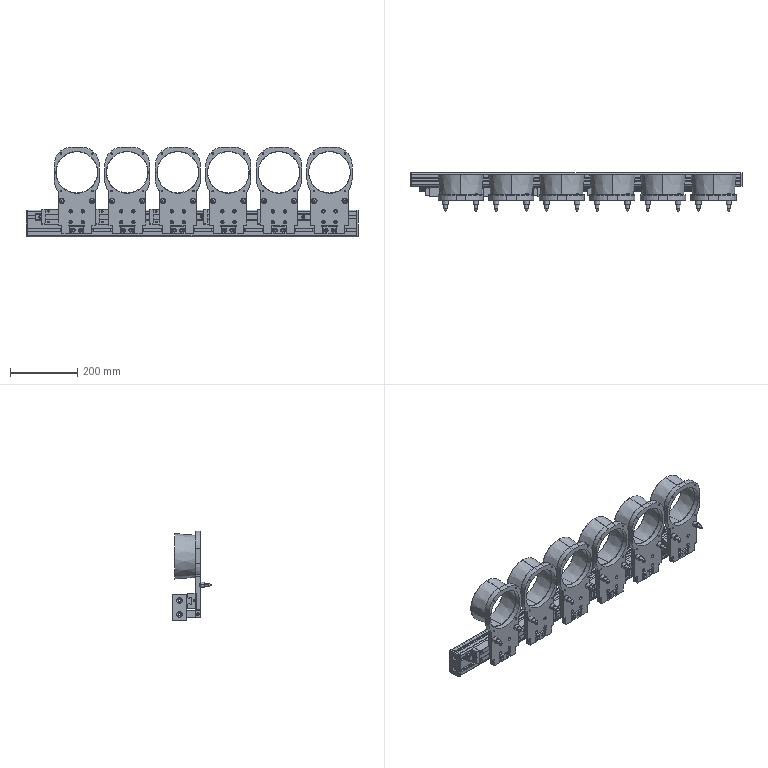Part | SolidWorks | 64 solids | 2142 faces | box 985 x 114 x 267 mm | volume 3601226 mm3 | plane 1040 | cylinder 818 | cone 260 | sphere 24 | commonest cylinder face diameters 5.5 x132 10 x96 4.2 x72 4.3 x48 7.4 x48 16 x48